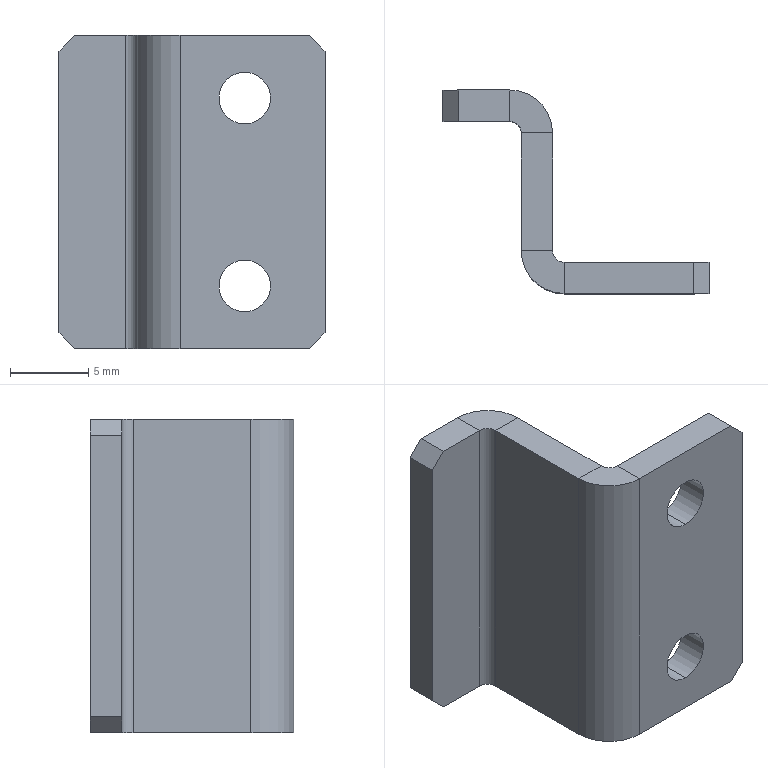Part | STEP file | 11-FG99-2015-7-17-S011-V3.0-kkkkkk-998.11 | 1 solid | 30 faces | box 17 x 13 x 20 mm | volume 1022 mm3 | plane 22 | cylinder 8 | commonest cylinder face diameters 3.3 x4 1.473 x2 5.473 x2
STEP:
#1=CARTESIAN_POINT('',(11.868,-11.,14.35));
#2=VERTEX_POINT('',#1);
#3=CARTESIAN_POINT('',(11.868,-11.,17.65));
#4=VERTEX_POINT('',#3);
#5=CARTESIAN_POINT('',(11.868,-11.,16.));
#6=DIRECTION('',(0.,1.,0.));
#7=DIRECTION('',(0.,0.,1.));
#8=AXIS2_PLACEMENT_3D('',#5,#6,#7);
#9=CIRCLE('',#8,1.65);
#10=EDGE_CURVE('',#2,#4,#9,.T.);
#11=ORIENTED_EDGE('',*,*,#10,.F.);
#12=CARTESIAN_POINT('',(11.868,-9.,14.35));
#13=VERTEX_POINT('',#12);
#14=CARTESIAN_POINT('',(11.868,-9.,14.35));
#15=DIRECTION('',(0.,1.,0.));
#16=VECTOR('',#15,1000.);
#17=LINE('',#14,#16);
#18=EDGE_CURVE('',#2,#13,#17,.T.);
#19=ORIENTED_EDGE('',*,*,#18,.T.);
#20=CARTESIAN_POINT('',(11.868,-9.,17.65));
#21=VERTEX_POINT('',#20);
#22=CARTESIAN_POINT('',(11.868,-9.,16.));
#23=DIRECTION('',(0.,1.,0.));
#24=DIRECTION('',(0.,0.,1.));
#25=AXIS2_PLACEMENT_3D('',#22,#23,#24);
#26=CIRCLE('',#25,1.65);
#27=EDGE_CURVE('',#13,#21,#26,.T.);
#28=ORIENTED_EDGE('',*,*,#27,.T.);
#29=CARTESIAN_POINT('',(11.868,-9.,17.65));
#30=DIRECTION('',(0.,1.,0.));
#31=VECTOR('',#30,1000.);
#32=LINE('',#29,#31);
#33=EDGE_CURVE('',#4,#21,#32,.T.);
#34=ORIENTED_EDGE('',*,*,#33,.F.);
#35=EDGE_LOOP('',(#11,#19,#28,#34));
#36=FACE_OUTER_BOUND('',#35,.T.);
#37=CARTESIAN_POINT('',(11.868,-9.,16.));
#38=DIRECTION('',(0.,1.,0.));
#39=DIRECTION('',(0.,0.,1.));
#40=AXIS2_PLACEMENT_3D('',#37,#38,#39);
#41=CYLINDRICAL_SURFACE('',#40,1.65);
#42=ADVANCED_FACE('',(#36),#41,.F.);
#43=CARTESIAN_POINT('',(11.868,-11.,2.35));
#44=VERTEX_POINT('',#43);
#45=CARTESIAN_POINT('',(11.868,-11.,5.65));
#46=VERTEX_POINT('',#45);
#47=CARTESIAN_POINT('',(11.868,-11.,4.));
#48=DIRECTION('',(0.,1.,0.));
#49=DIRECTION('',(0.,0.,1.));
#50=AXIS2_PLACEMENT_3D('',#47,#48,#49);
#51=CIRCLE('',#50,1.65);
#52=EDGE_CURVE('',#44,#46,#51,.T.);
#53=ORIENTED_EDGE('',*,*,#52,.F.);
#54=CARTESIAN_POINT('',(11.868,-9.,2.35));
#55=VERTEX_POINT('',#54);
#56=CARTESIAN_POINT('',(11.868,-9.,2.35));
#57=DIRECTION('',(0.,1.,0.));
#58=VECTOR('',#57,1000.);
#59=LINE('',#56,#58);
#60=EDGE_CURVE('',#44,#55,#59,.T.);
#61=ORIENTED_EDGE('',*,*,#60,.T.);
#62=CARTESIAN_POINT('',(11.868,-9.,5.65));
#63=VERTEX_POINT('',#62);
#64=CARTESIAN_POINT('',(11.868,-9.,4.));
#65=DIRECTION('',(0.,1.,0.));
#66=DIRECTION('',(0.,0.,1.));
#67=AXIS2_PLACEMENT_3D('',#64,#65,#66);
#68=CIRCLE('',#67,1.65);
#69=EDGE_CURVE('',#55,#63,#68,.T.);
#70=ORIENTED_EDGE('',*,*,#69,.T.);
#71=CARTESIAN_POINT('',(11.868,-9.,5.65));
#72=DIRECTION('',(0.,1.,0.));
#73=VECTOR('',#72,1000.);
#74=LINE('',#71,#73);
#75=EDGE_CURVE('',#46,#63,#74,.T.);
#76=ORIENTED_EDGE('',*,*,#75,.F.);
#77=EDGE_LOOP('',(#53,#61,#70,#76));
#78=FACE_OUTER_BOUND('',#77,.T.);
#79=CARTESIAN_POINT('',(11.868,-9.,4.));
#80=DIRECTION('',(0.,1.,0.));
#81=DIRECTION('',(0.,0.,1.));
#82=AXIS2_PLACEMENT_3D('',#79,#80,#81);
#83=CYLINDRICAL_SURFACE('',#82,1.65);
#84=ADVANCED_FACE('',(#78),#83,.F.);
#85=CARTESIAN_POINT('',(4.263,0.,20.));
#86=VERTEX_POINT('',#85);
#87=CARTESIAN_POINT('',(4.263,2.,20.));
#88=VERTEX_POINT('',#87);
#89=CARTESIAN_POINT('',(4.263,0.,20.));
#90=DIRECTION('',(0.,1.,0.));
#91=VECTOR('',#90,1000.);
#92=LINE('',#89,#91);
#93=EDGE_CURVE('',#86,#88,#92,.T.);
#94=ORIENTED_EDGE('',*,*,#93,.F.);
#95=CARTESIAN_POINT('',(5.,-0.7366,20.));
#96=VERTEX_POINT('',#95);
#97=CARTESIAN_POINT('',(4.263,-0.7366,20.));
#98=DIRECTION('',(0.,0.,-1.));
#99=DIRECTION('',(1.,0.,0.));
#100=AXIS2_PLACEMENT_3D('',#97,#98,#99);
#101=CIRCLE('',#100,0.7366);
#102=EDGE_CURVE('',#86,#96,#101,.T.);
#103=ORIENTED_EDGE('',*,*,#102,.T.);
#104=CARTESIAN_POINT('',(7.,-0.7366,20.));
#105=VERTEX_POINT('',#104);
#106=CARTESIAN_POINT('',(7.,-0.7366,20.));
#107=DIRECTION('',(-1.,0.,0.));
#108=VECTOR('',#107,1000.);
#109=LINE('',#106,#108);
#110=EDGE_CURVE('',#105,#96,#109,.T.);
#111=ORIENTED_EDGE('',*,*,#110,.F.);
#112=CARTESIAN_POINT('',(4.263,-0.7366,20.));
#113=DIRECTION('',(0.,0.,-1.));
#114=DIRECTION('',(1.,0.,0.));
#115=AXIS2_PLACEMENT_3D('',#112,#113,#114);
#116=CIRCLE('',#115,2.737);
#117=EDGE_CURVE('',#88,#105,#116,.T.);
#118=ORIENTED_EDGE('',*,*,#117,.F.);
#119=EDGE_LOOP('',(#94,#103,#111,#118));
#120=FACE_OUTER_BOUND('',#119,.T.);
#121=CARTESIAN_POINT('',(4.263,0.,20.));
#122=DIRECTION('',(0.,0.,1.));
#123=DIRECTION('',(1.,0.,0.));
#124=AXIS2_PLACEMENT_3D('',#121,#122,#123);
#125=PLANE('',#124);
#126=ADVANCED_FACE('',(#120),#125,.T.);
#127=CARTESIAN_POINT('',(1.,2.,20.));
#128=VERTEX_POINT('',#127);
#129=CARTESIAN_POINT('',(0.,2.,20.));
#130=DIRECTION('',(1.,0.,0.));
#131=VECTOR('',#130,1000.);
#132=LINE('',#129,#131);
#133=EDGE_CURVE('',#128,#88,#132,.T.);
#134=ORIENTED_EDGE('',*,*,#133,.F.);
#135=CARTESIAN_POINT('',(1.,0.,20.));
#136=VERTEX_POINT('',#135);
#137=CARTESIAN_POINT('',(1.,-0.7366,20.));
#138=DIRECTION('',(0.,-1.,0.));
#139=VECTOR('',#138,1000.);
#140=LINE('',#137,#139);
#141=EDGE_CURVE('',#128,#136,#140,.T.);
#142=ORIENTED_EDGE('',*,*,#141,.T.);
#143=CARTESIAN_POINT('',(0.,0.,20.));
#144=DIRECTION('',(1.,0.,0.));
#145=VECTOR('',#144,1000.);
#146=LINE('',#143,#145);
#147=EDGE_CURVE('',#136,#86,#146,.T.);
#148=ORIENTED_EDGE('',*,*,#147,.T.);
#149=ORIENTED_EDGE('',*,*,#93,.T.);
#150=EDGE_LOOP('',(#134,#142,#148,#149));
#151=FACE_OUTER_BOUND('',#150,.T.);
#152=CARTESIAN_POINT('',(7.,-0.7366,20.));
#153=DIRECTION('',(0.,0.,1.));
#154=DIRECTION('',(1.,0.,0.));
#155=AXIS2_PLACEMENT_3D('',#152,#153,#154);
#156=PLANE('',#155);
#157=ADVANCED_FACE('',(#151),#156,.T.);
#158=CARTESIAN_POINT('',(5.,-0.7366,0.));
#159=VERTEX_POINT('',#158);
#160=CARTESIAN_POINT('',(7.,-0.7366,0.));
#161=VERTEX_POINT('',#160);
#162=CARTESIAN_POINT('',(5.,-0.7366,0.));
#163=DIRECTION('',(1.,0.,0.));
#164=VECTOR('',#163,1000.);
#165=LINE('',#162,#164);
#166=EDGE_CURVE('',#159,#161,#165,.T.);
#167=ORIENTED_EDGE('',*,*,#166,.F.);
#168=CARTESIAN_POINT('',(4.263,0.,0.));
#169=VERTEX_POINT('',#168);
#170=CARTESIAN_POINT('',(4.263,-0.7366,0.));
#171=DIRECTION('',(0.,0.,-1.));
#172=DIRECTION('',(1.,0.,0.));
#173=AXIS2_PLACEMENT_3D('',#170,#171,#172);
#174=CIRCLE('',#173,0.7366);
#175=EDGE_CURVE('',#169,#159,#174,.T.);
#176=ORIENTED_EDGE('',*,*,#175,.F.);
#177=CARTESIAN_POINT('',(4.263,2.,0.));
#178=VERTEX_POINT('',#177);
#179=CARTESIAN_POINT('',(4.263,2.,0.));
#180=DIRECTION('',(0.,-1.,0.));
#181=VECTOR('',#180,1000.);
#182=LINE('',#179,#181);
#183=EDGE_CURVE('',#178,#169,#182,.T.);
#184=ORIENTED_EDGE('',*,*,#183,.F.);
#185=CARTESIAN_POINT('',(4.263,-0.7366,0.));
#186=DIRECTION('',(0.,0.,-1.));
#187=DIRECTION('',(1.,0.,0.));
#188=AXIS2_PLACEMENT_3D('',#185,#186,#187);
#189=CIRCLE('',#188,2.737);
#190=EDGE_CURVE('',#178,#161,#189,.T.);
#191=ORIENTED_EDGE('',*,*,#190,.T.);
#192=EDGE_LOOP('',(#167,#176,#184,#191));
#193=FACE_OUTER_BOUND('',#192,.T.);
#194=CARTESIAN_POINT('',(5.,-0.7366,0.));
#195=DIRECTION('',(0.,0.,-1.));
#196=DIRECTION('',(-1.,0.,0.));
#197=AXIS2_PLACEMENT_3D('',#194,#195,#196);
#198=PLANE('',#197);
#199=ADVANCED_FACE('',(#193),#198,.T.);
#200=CARTESIAN_POINT('',(5.,-8.263,0.));
#201=VERTEX_POINT('',#200);
#202=CARTESIAN_POINT('',(5.,0.,0.));
#203=DIRECTION('',(0.,-1.,0.));
#204=VECTOR('',#203,1000.);
#205=LINE('',#202,#204);
#206=EDGE_CURVE('',#159,#201,#205,.T.);
#207=ORIENTED_EDGE('',*,*,#206,.F.);
#208=ORIENTED_EDGE('',*,*,#166,.T.);
#209=CARTESIAN_POINT('',(7.,-8.263,0.));
#210=VERTEX_POINT('',#209);
#211=CARTESIAN_POINT('',(7.,0.,0.));
#212=DIRECTION('',(0.,-1.,0.));
#213=VECTOR('',#212,1000.);
#214=LINE('',#211,#213);
#215=EDGE_CURVE('',#161,#210,#214,.T.);
#216=ORIENTED_EDGE('',*,*,#215,.T.);
#217=CARTESIAN_POINT('',(7.,-8.263,0.));
#218=DIRECTION('',(-1.,0.,0.));
#219=VECTOR('',#218,1000.);
#220=LINE('',#217,#219);
#221=EDGE_CURVE('',#210,#201,#220,.T.);
#222=ORIENTED_EDGE('',*,*,#221,.T.);
#223=EDGE_LOOP('',(#207,#208,#216,#222));
#224=FACE_OUTER_BOUND('',#223,.T.);
#225=CARTESIAN_POINT('',(4.263,2.,0.));
#226=DIRECTION('',(0.,0.,-1.));
#227=DIRECTION('',(-1.,0.,0.));
#228=AXIS2_PLACEMENT_3D('',#225,#226,#227);
#229=PLANE('',#228);
#230=ADVANCED_FACE('',(#224),#229,.T.);
#231=CARTESIAN_POINT('',(5.,-8.263,20.));
#232=VERTEX_POINT('',#231);
#233=CARTESIAN_POINT('',(7.,-8.263,20.));
#234=VERTEX_POINT('',#233);
#235=CARTESIAN_POINT('',(5.,-8.263,20.));
#236=DIRECTION('',(1.,0.,0.));
#237=VECTOR('',#236,1000.);
#238=LINE('',#235,#237);
#239=EDGE_CURVE('',#232,#234,#238,.T.);
#240=ORIENTED_EDGE('',*,*,#239,.F.);
#241=CARTESIAN_POINT('',(7.737,-11.,20.));
#242=VERTEX_POINT('',#241);
#243=CARTESIAN_POINT('',(7.737,-8.263,20.));
#244=DIRECTION('',(0.,0.,1.));
#245=DIRECTION('',(-1.,0.,0.));
#246=AXIS2_PLACEMENT_3D('',#243,#244,#245);
#247=CIRCLE('',#246,2.737);
#248=EDGE_CURVE('',#232,#242,#247,.T.);
#249=ORIENTED_EDGE('',*,*,#248,.T.);
#250=CARTESIAN_POINT('',(7.737,-9.,20.));
#251=VERTEX_POINT('',#250);
#252=CARTESIAN_POINT('',(7.737,-9.,20.));
#253=DIRECTION('',(0.,-1.,0.));
#254=VECTOR('',#253,1000.);
#255=LINE('',#252,#254);
#256=EDGE_CURVE('',#251,#242,#255,.T.);
#257=ORIENTED_EDGE('',*,*,#256,.F.);
#258=CARTESIAN_POINT('',(7.737,-8.263,20.));
#259=DIRECTION('',(0.,0.,1.));
#260=DIRECTION('',(1.,0.,0.));
#261=AXIS2_PLACEMENT_3D('',#258,#259,#260);
#262=CIRCLE('',#261,0.7366);
#263=EDGE_CURVE('',#234,#251,#262,.T.);
#264=ORIENTED_EDGE('',*,*,#263,.F.);
#265=EDGE_LOOP('',(#240,#249,#257,#264));
#266=FACE_OUTER_BOUND('',#265,.T.);
#267=CARTESIAN_POINT('',(5.,-8.263,20.));
#268=DIRECTION('',(0.,0.,1.));
#269=DIRECTION('',(1.,0.,0.));
#270=AXIS2_PLACEMENT_3D('',#267,#268,#269);
#271=PLANE('',#270);
#272=ADVANCED_FACE('',(#266),#271,.T.);
#273=CARTESIAN_POINT('',(5.,0.,20.));
#274=DIRECTION('',(0.,-1.,0.));
#275=VECTOR('',#274,1000.);
#276=LINE('',#273,#275);
#277=EDGE_CURVE('',#96,#232,#276,.T.);
#278=ORIENTED_EDGE('',*,*,#277,.T.);
#279=ORIENTED_EDGE('',*,*,#239,.T.);
#280=CARTESIAN_POINT('',(7.,0.,20.));
#281=DIRECTION('',(0.,-1.,0.));
#282=VECTOR('',#281,1000.);
#283=LINE('',#280,#282);
#284=EDGE_CURVE('',#105,#234,#283,.T.);
#285=ORIENTED_EDGE('',*,*,#284,.F.);
#286=ORIENTED_EDGE('',*,*,#110,.T.);
#287=EDGE_LOOP('',(#278,#279,#285,#286));
#288=FACE_OUTER_BOUND('',#287,.T.);
#289=CARTESIAN_POINT('',(7.737,-9.,20.));
#290=DIRECTION('',(0.,0.,1.));
#291=DIRECTION('',(1.,0.,0.));
#292=AXIS2_PLACEMENT_3D('',#289,#290,#291);
#293=PLANE('',#292);
#294=ADVANCED_FACE('',(#288),#293,.T.);
#295=CARTESIAN_POINT('',(7.737,-11.,0.));
#296=VERTEX_POINT('',#295);
#297=CARTESIAN_POINT('',(7.737,-9.,0.));
#298=VERTEX_POINT('',#297);
#299=CARTESIAN_POINT('',(7.737,-11.,0.));
#300=DIRECTION('',(0.,1.,0.));
#301=VECTOR('',#300,1000.);
#302=LINE('',#299,#301);
#303=EDGE_CURVE('',#296,#298,#302,.T.);
#304=ORIENTED_EDGE('',*,*,#303,.F.);
#305=CARTESIAN_POINT('',(7.737,-8.263,0.));
#306=DIRECTION('',(0.,0.,1.));
#307=DIRECTION('',(-1.,0.,0.));
#308=AXIS2_PLACEMENT_3D('',#305,#306,#307);
#309=CIRCLE('',#308,2.737);
#310=EDGE_CURVE('',#201,#296,#309,.T.);
#311=ORIENTED_EDGE('',*,*,#310,.F.);
#312=ORIENTED_EDGE('',*,*,#221,.F.);
#313=CARTESIAN_POINT('',(7.737,-8.263,0.));
#314=DIRECTION('',(0.,0.,1.));
#315=DIRECTION('',(1.,0.,0.));
#316=AXIS2_PLACEMENT_3D('',#313,#314,#315);
#317=CIRCLE('',#316,0.7366);
#318=EDGE_CURVE('',#210,#298,#317,.T.);
#319=ORIENTED_EDGE('',*,*,#318,.T.);
#320=EDGE_LOOP('',(#304,#311,#312,#319));
#321=FACE_OUTER_BOUND('',#320,.T.);
#322=CARTESIAN_POINT('',(7.737,-11.,0.));
#323=DIRECTION('',(0.,0.,-1.));
#324=DIRECTION('',(-1.,0.,0.));
#325=AXIS2_PLACEMENT_3D('',#322,#323,#324);
#326=PLANE('',#325);
#327=ADVANCED_FACE('',(#321),#326,.T.);
#328=CARTESIAN_POINT('',(16.,-9.,0.));
#329=VERTEX_POINT('',#328);
#330=CARTESIAN_POINT('',(5.,-9.,0.));
#331=DIRECTION('',(1.,0.,0.));
#332=VECTOR('',#331,1000.);
#333=LINE('',#330,#332);
#334=EDGE_CURVE('',#298,#329,#333,.T.);
#335=ORIENTED_EDGE('',*,*,#334,.T.);
#336=CARTESIAN_POINT('',(16.,-11.,0.));
#337=VERTEX_POINT('',#336);
#338=CARTESIAN_POINT('',(16.,-8.263,0.));
#339=DIRECTION('',(0.,-1.,0.));
#340=VECTOR('',#339,1000.);
#341=LINE('',#338,#340);
#342=EDGE_CURVE('',#329,#337,#341,.T.);
#343=ORIENTED_EDGE('',*,*,#342,.T.);
#344=CARTESIAN_POINT('',(5.,-11.,0.));
#345=DIRECTION('',(1.,0.,0.));
#346=VECTOR('',#345,1000.);
#347=LINE('',#344,#346);
#348=EDGE_CURVE('',#296,#337,#347,.T.);
#349=ORIENTED_EDGE('',*,*,#348,.F.);
#350=ORIENTED_EDGE('',*,*,#303,.T.);
#351=EDGE_LOOP('',(#335,#343,#349,#350));
#352=FACE_OUTER_BOUND('',#351,.T.);
#353=CARTESIAN_POINT('',(7.,-8.263,0.));
#354=DIRECTION('',(0.,0.,-1.));
#355=DIRECTION('',(-1.,0.,0.));
#356=AXIS2_PLACEMENT_3D('',#353,#354,#355);
#357=PLANE('',#356);
#358=ADVANCED_FACE('',(#352),#357,.T.);
#359=CARTESIAN_POINT('',(11.868,-11.,16.));
#360=DIRECTION('',(0.,1.,0.));
#361=DIRECTION('',(0.,0.,1.));
#362=AXIS2_PLACEMENT_3D('',#359,#360,#361);
#363=CIRCLE('',#362,1.65);
#364=EDGE_CURVE('',#4,#2,#363,.T.);
#365=ORIENTED_EDGE('',*,*,#364,.T.);
#366=ORIENTED_EDGE('',*,*,#10,.T.);
#367=EDGE_LOOP('',(#365,#366));
#368=FACE_BOUND('',#367,.T.);
#369=CARTESIAN_POINT('',(11.868,-11.,4.));
#370=DIRECTION('',(0.,1.,0.));
#371=DIRECTION('',(0.,0.,1.));
#372=AXIS2_PLACEMENT_3D('',#369,#370,#371);
#373=CIRCLE('',#372,1.65);
#374=EDGE_CURVE('',#46,#44,#373,.T.);
#375=ORIENTED_EDGE('',*,*,#374,.T.);
#376=ORIENTED_EDGE('',*,*,#52,.T.);
#377=EDGE_LOOP('',(#375,#376));
#378=FACE_BOUND('',#377,.T.);
#379=ORIENTED_EDGE('',*,*,#348,.T.);
#380=CARTESIAN_POINT('',(17.,-11.,1.));
#381=VERTEX_POINT('',#380);
#382=CARTESIAN_POINT('',(16.,-11.,0.));
#383=DIRECTION('',(0.7071,0.,0.7071));
#384=VECTOR('',#383,1000.);
#385=LINE('',#382,#384);
#386=EDGE_CURVE('',#337,#381,#385,.T.);
#387=ORIENTED_EDGE('',*,*,#386,.T.);
#388=CARTESIAN_POINT('',(17.,-11.,19.));
#389=VERTEX_POINT('',#388);
#390=CARTESIAN_POINT('',(17.,-11.,20.));
#391=DIRECTION('',(0.,0.,-1.));
#392=VECTOR('',#391,1000.);
#393=LINE('',#390,#392);
#394=EDGE_CURVE('',#389,#381,#393,.T.);
#395=ORIENTED_EDGE('',*,*,#394,.F.);
#396=CARTESIAN_POINT('',(16.,-11.,20.));
#397=VERTEX_POINT('',#396);
#398=CARTESIAN_POINT('',(17.,-11.,19.));
#399=DIRECTION('',(-0.7071,0.,0.7071));
#400=VECTOR('',#399,1000.);
#401=LINE('',#398,#400);
#402=EDGE_CURVE('',#389,#397,#401,.T.);
#403=ORIENTED_EDGE('',*,*,#402,.T.);
#404=CARTESIAN_POINT('',(5.,-11.,20.));
#405=DIRECTION('',(1.,0.,0.));
#406=VECTOR('',#405,1000.);
#407=LINE('',#404,#406);
#408=EDGE_CURVE('',#242,#397,#407,.T.);
#409=ORIENTED_EDGE('',*,*,#408,.F.);
#410=CARTESIAN_POINT('',(7.737,-11.,20.));
#411=DIRECTION('',(0.,0.,-1.));
#412=VECTOR('',#411,1000.);
#413=LINE('',#410,#412);
#414=EDGE_CURVE('',#242,#296,#413,.T.);
#415=ORIENTED_EDGE('',*,*,#414,.T.);
#416=EDGE_LOOP('',(#379,#387,#395,#403,#409,#415));
#417=FACE_OUTER_BOUND('',#416,.T.);
#418=CARTESIAN_POINT('',(5.,-11.,20.));
#419=DIRECTION('',(0.,1.,0.));
#420=DIRECTION('',(0.,0.,1.));
#421=AXIS2_PLACEMENT_3D('',#418,#419,#420);
#422=PLANE('',#421);
#423=ADVANCED_FACE('',(#368,#378,#417),#422,.F.);
#424=ORIENTED_EDGE('',*,*,#394,.T.);
#425=CARTESIAN_POINT('',(17.,-9.,1.));
#426=VERTEX_POINT('',#425);
#427=CARTESIAN_POINT('',(17.,-9.,1.));
#428=DIRECTION('',(0.,1.,0.));
#429=VECTOR('',#428,1000.);
#430=LINE('',#427,#429);
#431=EDGE_CURVE('',#381,#426,#430,.T.);
#432=ORIENTED_EDGE('',*,*,#431,.T.);
#433=CARTESIAN_POINT('',(17.,-9.,19.));
#434=VERTEX_POINT('',#433);
#435=CARTESIAN_POINT('',(17.,-9.,20.));
#436=DIRECTION('',(0.,0.,-1.));
#437=VECTOR('',#436,1000.);
#438=LINE('',#435,#437);
#439=EDGE_CURVE('',#434,#426,#438,.T.);
#440=ORIENTED_EDGE('',*,*,#439,.F.);
#441=CARTESIAN_POINT('',(17.,-9.,19.));
#442=DIRECTION('',(0.,-1.,0.));
#443=VECTOR('',#442,1000.);
#444=LINE('',#441,#443);
#445=EDGE_CURVE('',#434,#389,#444,.T.);
#446=ORIENTED_EDGE('',*,*,#445,.T.);
#447=EDGE_LOOP('',(#424,#432,#440,#446));
#448=FACE_OUTER_BOUND('',#447,.T.);
#449=CARTESIAN_POINT('',(17.,-9.,20.));
#450=DIRECTION('',(1.,0.,0.));
#451=DIRECTION('',(0.,0.,-1.));
#452=AXIS2_PLACEMENT_3D('',#449,#450,#451);
#453=PLANE('',#452);
#454=ADVANCED_FACE('',(#448),#453,.T.);
#455=CARTESIAN_POINT('',(11.868,-9.,16.));
#456=DIRECTION('',(0.,1.,0.));
#457=DIRECTION('',(0.,0.,1.));
#458=AXIS2_PLACEMENT_3D('',#455,#456,#457);
#459=CIRCLE('',#458,1.65);
#460=EDGE_CURVE('',#21,#13,#459,.T.);
#461=ORIENTED_EDGE('',*,*,#460,.F.);
#462=ORIENTED_EDGE('',*,*,#27,.F.);
#463=EDGE_LOOP('',(#461,#462));
#464=FACE_BOUND('',#463,.T.);
#465=CARTESIAN_POINT('',(11.868,-9.,4.));
#466=DIRECTION('',(0.,1.,0.));
#467=DIRECTION('',(0.,0.,1.));
#468=AXIS2_PLACEMENT_3D('',#465,#466,#467);
#469=CIRCLE('',#468,1.65);
#470=EDGE_CURVE('',#63,#55,#469,.T.);
#471=ORIENTED_EDGE('',*,*,#470,.F.);
#472=ORIENTED_EDGE('',*,*,#69,.F.);
#473=EDGE_LOOP('',(#471,#472));
#474=FACE_BOUND('',#473,.T.);
#475=ORIENTED_EDGE('',*,*,#439,.T.);
#476=CARTESIAN_POINT('',(20.5,-9.,4.5));
#477=DIRECTION('',(-0.7071,0.,-0.7071));
#478=VECTOR('',#477,1000.);
#479=LINE('',#476,#478);
#480=EDGE_CURVE('',#426,#329,#479,.T.);
#481=ORIENTED_EDGE('',*,*,#480,.T.);
#482=ORIENTED_EDGE('',*,*,#334,.F.);
#483=CARTESIAN_POINT('',(7.737,-9.,20.));
#484=DIRECTION('',(0.,0.,-1.));
#485=VECTOR('',#484,1000.);
#486=LINE('',#483,#485);
#487=EDGE_CURVE('',#251,#298,#486,.T.);
#488=ORIENTED_EDGE('',*,*,#487,.F.);
#489=CARTESIAN_POINT('',(16.,-9.,20.));
#490=VERTEX_POINT('',#489);
#491=CARTESIAN_POINT('',(5.,-9.,20.));
#492=DIRECTION('',(1.,0.,0.));
#493=VECTOR('',#492,1000.);
#494=LINE('',#491,#493);
#495=EDGE_CURVE('',#251,#490,#494,.T.);
#496=ORIENTED_EDGE('',*,*,#495,.T.);
#497=CARTESIAN_POINT('',(10.5,-9.,25.5));
#498=DIRECTION('',(0.7071,0.,-0.7071));
#499=VECTOR('',#498,1000.);
#500=LINE('',#497,#499);
#501=EDGE_CURVE('',#490,#434,#500,.T.);
#502=ORIENTED_EDGE('',*,*,#501,.T.);
#503=EDGE_LOOP('',(#475,#481,#482,#488,#496,#502));
#504=FACE_OUTER_BOUND('',#503,.T.);
#505=CARTESIAN_POINT('',(5.,-9.,20.));
#506=DIRECTION('',(0.,1.,0.));
#507=DIRECTION('',(0.,0.,1.));
#508=AXIS2_PLACEMENT_3D('',#505,#506,#507);
#509=PLANE('',#508);
#510=ADVANCED_FACE('',(#464,#474,#504),#509,.T.);
#511=ORIENTED_EDGE('',*,*,#318,.F.);
#512=CARTESIAN_POINT('',(7.,-8.263,20.));
#513=DIRECTION('',(0.,0.,-1.));
#514=VECTOR('',#513,1000.);
#515=LINE('',#512,#514);
#516=EDGE_CURVE('',#234,#210,#515,.T.);
#517=ORIENTED_EDGE('',*,*,#516,.F.);
#518=ORIENTED_EDGE('',*,*,#263,.T.);
#519=ORIENTED_EDGE('',*,*,#487,.T.);
#520=EDGE_LOOP('',(#511,#517,#518,#519));
#521=FACE_OUTER_BOUND('',#520,.T.);
#522=CARTESIAN_POINT('',(7.737,-8.263,20.));
#523=DIRECTION('',(0.,0.,-1.));
#524=DIRECTION('',(-1.,0.,0.));
#525=AXIS2_PLACEMENT_3D('',#522,#523,#524);
#526=CYLINDRICAL_SURFACE('',#525,0.7366);
#527=ADVANCED_FACE('',(#521),#526,.F.);
#528=ORIENTED_EDGE('',*,*,#215,.F.);
#529=CARTESIAN_POINT('',(7.,-0.7366,20.));
#530=DIRECTION('',(0.,0.,-1.));
#531=VECTOR('',#530,1000.);
#532=LINE('',#529,#531);
#533=EDGE_CURVE('',#105,#161,#532,.T.);
#534=ORIENTED_EDGE('',*,*,#533,.F.);
#535=ORIENTED_EDGE('',*,*,#284,.T.);
#536=ORIENTED_EDGE('',*,*,#516,.T.);
#537=EDGE_LOOP('',(#528,#534,#535,#536));
#538=FACE_OUTER_BOUND('',#537,.T.);
#539=CARTESIAN_POINT('',(7.,0.,20.));
#540=DIRECTION('',(1.,0.,0.));
#541=DIRECTION('',(0.,1.,0.));
#542=AXIS2_PLACEMENT_3D('',#539,#540,#541);
#543=PLANE('',#542);
#544=ADVANCED_FACE('',(#538),#543,.T.);
#545=ORIENTED_EDGE('',*,*,#190,.F.);
#546=CARTESIAN_POINT('',(4.263,2.,20.));
#547=DIRECTION('',(0.,0.,-1.));
#548=VECTOR('',#547,1000.);
#549=LINE('',#546,#548);
#550=EDGE_CURVE('',#88,#178,#549,.T.);
#551=ORIENTED_EDGE('',*,*,#550,.F.);
#552=ORIENTED_EDGE('',*,*,#117,.T.);
#553=ORIENTED_EDGE('',*,*,#533,.T.);
#554=EDGE_LOOP('',(#545,#551,#552,#553));
#555=FACE_OUTER_BOUND('',#554,.T.);
#556=CARTESIAN_POINT('',(4.263,-0.7366,20.));
#557=DIRECTION('',(0.,0.,-1.));
#558=DIRECTION('',(-1.,0.,0.));
#559=AXIS2_PLACEMENT_3D('',#556,#557,#558);
#560=CYLINDRICAL_SURFACE('',#559,2.737);
#561=ADVANCED_FACE('',(#555),#560,.T.);
#562=CARTESIAN_POINT('',(1.,2.,0.));
#563=VERTEX_POINT('',#562);
#564=CARTESIAN_POINT('',(0.,2.,0.));
#565=DIRECTION('',(1.,0.,0.));
#566=VECTOR('',#565,1000.);
#567=LINE('',#564,#566);
#568=EDGE_CURVE('',#563,#178,#567,.T.);
#569=ORIENTED_EDGE('',*,*,#568,.F.);
#570=CARTESIAN_POINT('',(0.,2.,1.));
#571=VERTEX_POINT('',#570);
#572=CARTESIAN_POINT('',(-9.5,2.,10.5));
#573=DIRECTION('',(-0.7071,0.,0.7071));
#574=VECTOR('',#573,1000.);
#575=LINE('',#572,#574);
#576=EDGE_CURVE('',#563,#571,#575,.T.);
#577=ORIENTED_EDGE('',*,*,#576,.T.);
#578=CARTESIAN_POINT('',(0.,2.,19.));
#579=VERTEX_POINT('',#578);
#580=CARTESIAN_POINT('',(0.,2.,20.));
#581=DIRECTION('',(0.,0.,-1.));
#582=VECTOR('',#581,1000.);
#583=LINE('',#580,#582);
#584=EDGE_CURVE('',#579,#571,#583,.T.);
#585=ORIENTED_EDGE('',*,*,#584,.F.);
#586=CARTESIAN_POINT('',(0.5,2.,19.5));
#587=DIRECTION('',(0.7071,0.,0.7071));
#588=VECTOR('',#587,1000.);
#589=LINE('',#586,#588);
#590=EDGE_CURVE('',#579,#128,#589,.T.);
#591=ORIENTED_EDGE('',*,*,#590,.T.);
#592=ORIENTED_EDGE('',*,*,#133,.T.);
#593=ORIENTED_EDGE('',*,*,#550,.T.);
#594=EDGE_LOOP('',(#569,#577,#585,#591,#592,#593));
#595=FACE_OUTER_BOUND('',#594,.T.);
#596=CARTESIAN_POINT('',(0.,2.,20.));
#597=DIRECTION('',(0.,1.,0.));
#598=DIRECTION('',(0.,0.,1.));
#599=AXIS2_PLACEMENT_3D('',#596,#597,#598);
#600=PLANE('',#599);
#601=ADVANCED_FACE('',(#595),#600,.T.);
#602=ORIENTED_EDGE('',*,*,#584,.T.);
#603=CARTESIAN_POINT('',(0.,0.,1.));
#604=VERTEX_POINT('',#603);
#605=CARTESIAN_POINT('',(0.,0.,1.));
#606=DIRECTION('',(0.,-1.,0.));
#607=VECTOR('',#606,1000.);
#608=LINE('',#605,#607);
#609=EDGE_CURVE('',#571,#604,#608,.T.);
#610=ORIENTED_EDGE('',*,*,#609,.T.);
#611=CARTESIAN_POINT('',(0.,0.,19.));
#612=VERTEX_POINT('',#611);
#613=CARTESIAN_POINT('',(0.,0.,20.));
#614=DIRECTION('',(0.,0.,-1.));
#615=VECTOR('',#614,1000.);
#616=LINE('',#613,#615);
#617=EDGE_CURVE('',#612,#604,#616,.T.);
#618=ORIENTED_EDGE('',*,*,#617,.F.);
#619=CARTESIAN_POINT('',(0.,0.,19.));
#620=DIRECTION('',(0.,1.,0.));
#621=VECTOR('',#620,1000.);
#622=LINE('',#619,#621);
#623=EDGE_CURVE('',#612,#579,#622,.T.);
#624=ORIENTED_EDGE('',*,*,#623,.T.);
#625=EDGE_LOOP('',(#602,#610,#618,#624));
#626=FACE_OUTER_BOUND('',#625,.T.);
#627=CARTESIAN_POINT('',(0.,0.,20.));
#628=DIRECTION('',(-1.,0.,0.));
#629=DIRECTION('',(0.,0.,1.));
#630=AXIS2_PLACEMENT_3D('',#627,#628,#629);
#631=PLANE('',#630);
#632=ADVANCED_FACE('',(#626),#631,.T.);
#633=ORIENTED_EDGE('',*,*,#617,.T.);
#634=CARTESIAN_POINT('',(1.,0.,0.));
#635=VERTEX_POINT('',#634);
#636=CARTESIAN_POINT('',(1.,0.,0.));
#637=DIRECTION('',(0.7071,0.,-0.7071));
#638=VECTOR('',#637,1000.);
#639=LINE('',#636,#638);
#640=EDGE_CURVE('',#604,#635,#639,.T.);
#641=ORIENTED_EDGE('',*,*,#640,.T.);
#642=CARTESIAN_POINT('',(0.,0.,0.));
#643=DIRECTION('',(1.,0.,0.));
#644=VECTOR('',#643,1000.);
#645=LINE('',#642,#644);
#646=EDGE_CURVE('',#635,#169,#645,.T.);
#647=ORIENTED_EDGE('',*,*,#646,.T.);
#648=CARTESIAN_POINT('',(4.263,0.,20.));
#649=DIRECTION('',(0.,0.,-1.));
#650=VECTOR('',#649,1000.);
#651=LINE('',#648,#650);
#652=EDGE_CURVE('',#86,#169,#651,.T.);
#653=ORIENTED_EDGE('',*,*,#652,.F.);
#654=ORIENTED_EDGE('',*,*,#147,.F.);
#655=CARTESIAN_POINT('',(0.,0.,19.));
#656=DIRECTION('',(-0.7071,0.,-0.7071));
#657=VECTOR('',#656,1000.);
#658=LINE('',#655,#657);
#659=EDGE_CURVE('',#136,#612,#658,.T.);
#660=ORIENTED_EDGE('',*,*,#659,.T.);
#661=EDGE_LOOP('',(#633,#641,#647,#653,#654,#660));
#662=FACE_OUTER_BOUND('',#661,.T.);
#663=CARTESIAN_POINT('',(0.,0.,20.));
#664=DIRECTION('',(0.,1.,0.));
#665=DIRECTION('',(0.,0.,1.));
#666=AXIS2_PLACEMENT_3D('',#663,#664,#665);
#667=PLANE('',#666);
#668=ADVANCED_FACE('',(#662),#667,.F.);
#669=ORIENTED_EDGE('',*,*,#175,.T.);
#670=CARTESIAN_POINT('',(5.,-0.7366,20.));
#671=DIRECTION('',(0.,0.,-1.));
#672=VECTOR('',#671,1000.);
#673=LINE('',#670,#672);
#674=EDGE_CURVE('',#96,#159,#673,.T.);
#675=ORIENTED_EDGE('',*,*,#674,.F.);
#676=ORIENTED_EDGE('',*,*,#102,.F.);
#677=ORIENTED_EDGE('',*,*,#652,.T.);
#678=EDGE_LOOP('',(#669,#675,#676,#677));
#679=FACE_OUTER_BOUND('',#678,.T.);
#680=CARTESIAN_POINT('',(4.263,-0.7366,20.));
#681=DIRECTION('',(0.,0.,-1.));
#682=DIRECTION('',(-1.,0.,0.));
#683=AXIS2_PLACEMENT_3D('',#680,#681,#682);
#684=CYLINDRICAL_SURFACE('',#683,0.7366);
#685=ADVANCED_FACE('',(#679),#684,.F.);
#686=ORIENTED_EDGE('',*,*,#206,.T.);
#687=CARTESIAN_POINT('',(5.,-8.263,20.));
#688=DIRECTION('',(0.,0.,-1.));
#689=VECTOR('',#688,1000.);
#690=LINE('',#687,#689);
#691=EDGE_CURVE('',#232,#201,#690,.T.);
#692=ORIENTED_EDGE('',*,*,#691,.F.);
#693=ORIENTED_EDGE('',*,*,#277,.F.);
#694=ORIENTED_EDGE('',*,*,#674,.T.);
#695=EDGE_LOOP('',(#686,#692,#693,#694));
#696=FACE_OUTER_BOUND('',#695,.T.);
#697=CARTESIAN_POINT('',(5.,0.,20.));
#698=DIRECTION('',(1.,0.,0.));
#699=DIRECTION('',(0.,1.,0.));
#700=AXIS2_PLACEMENT_3D('',#697,#698,#699);
#701=PLANE('',#700);
#702=ADVANCED_FACE('',(#696),#701,.F.);
#703=ORIENTED_EDGE('',*,*,#310,.T.);
#704=ORIENTED_EDGE('',*,*,#414,.F.);
#705=ORIENTED_EDGE('',*,*,#248,.F.);
#706=ORIENTED_EDGE('',*,*,#691,.T.);
#707=EDGE_LOOP('',(#703,#704,#705,#706));
#708=FACE_OUTER_BOUND('',#707,.T.);
#709=CARTESIAN_POINT('',(7.737,-8.263,20.));
#710=DIRECTION('',(0.,0.,-1.));
#711=DIRECTION('',(-1.,0.,0.));
#712=AXIS2_PLACEMENT_3D('',#709,#710,#711);
#713=CYLINDRICAL_SURFACE('',#712,2.737);
#714=ADVANCED_FACE('',(#708),#713,.T.);
#715=ORIENTED_EDGE('',*,*,#408,.T.);
#716=CARTESIAN_POINT('',(16.,-8.263,20.));
#717=DIRECTION('',(0.,1.,0.));
#718=VECTOR('',#717,1000.);
#719=LINE('',#716,#718);
#720=EDGE_CURVE('',#397,#490,#719,.T.);
#721=ORIENTED_EDGE('',*,*,#720,.T.);
#722=ORIENTED_EDGE('',*,*,#495,.F.);
#723=ORIENTED_EDGE('',*,*,#256,.T.);
#724=EDGE_LOOP('',(#715,#721,#722,#723));
#725=FACE_OUTER_BOUND('',#724,.T.);
#726=CARTESIAN_POINT('',(7.737,-8.263,20.));
#727=DIRECTION('',(0.,0.,1.));
#728=DIRECTION('',(1.,0.,0.));
#729=AXIS2_PLACEMENT_3D('',#726,#727,#728);
#730=PLANE('',#729);
#731=ADVANCED_FACE('',(#725),#730,.T.);
#732=ORIENTED_EDGE('',*,*,#646,.F.);
#733=CARTESIAN_POINT('',(1.,2.,0.));
#734=DIRECTION('',(0.,1.,0.));
#735=VECTOR('',#734,1000.);
#736=LINE('',#733,#735);
#737=EDGE_CURVE('',#635,#563,#736,.T.);
#738=ORIENTED_EDGE('',*,*,#737,.T.);
#739=ORIENTED_EDGE('',*,*,#568,.T.);
#740=ORIENTED_EDGE('',*,*,#183,.T.);
#741=EDGE_LOOP('',(#732,#738,#739,#740));
#742=FACE_OUTER_BOUND('',#741,.T.);
#743=CARTESIAN_POINT('',(7.737,-8.263,0.));
#744=DIRECTION('',(0.,0.,1.));
#745=DIRECTION('',(1.,0.,0.));
#746=AXIS2_PLACEMENT_3D('',#743,#744,#745);
#747=PLANE('',#746);
#748=ADVANCED_FACE('',(#742),#747,.F.);
#749=ORIENTED_EDGE('',*,*,#640,.F.);
#750=ORIENTED_EDGE('',*,*,#609,.F.);
#751=ORIENTED_EDGE('',*,*,#576,.F.);
#752=ORIENTED_EDGE('',*,*,#737,.F.);
#753=EDGE_LOOP('',(#749,#750,#751,#752));
#754=FACE_OUTER_BOUND('',#753,.T.);
#755=CARTESIAN_POINT('',(1.,-8.263,0.));
#756=DIRECTION('',(-0.7071,0.,-0.7071));
#757=DIRECTION('',(0.,-1.,0.));
#758=AXIS2_PLACEMENT_3D('',#755,#756,#757);
#759=PLANE('',#758);
#760=ADVANCED_FACE('',(#754),#759,.T.);
#761=ORIENTED_EDGE('',*,*,#659,.F.);
#762=ORIENTED_EDGE('',*,*,#141,.F.);
#763=ORIENTED_EDGE('',*,*,#590,.F.);
#764=ORIENTED_EDGE('',*,*,#623,.F.);
#765=EDGE_LOOP('',(#761,#762,#763,#764));
#766=FACE_OUTER_BOUND('',#765,.T.);
#767=CARTESIAN_POINT('',(0.,0.,19.));
#768=DIRECTION('',(0.7071,0.,-0.7071));
#769=DIRECTION('',(0.,1.,0.));
#770=AXIS2_PLACEMENT_3D('',#767,#768,#769);
#771=PLANE('',#770);
#772=ADVANCED_FACE('',(#766),#771,.F.);
#773=ORIENTED_EDGE('',*,*,#480,.F.);
#774=ORIENTED_EDGE('',*,*,#431,.F.);
#775=ORIENTED_EDGE('',*,*,#386,.F.);
#776=ORIENTED_EDGE('',*,*,#342,.F.);
#777=EDGE_LOOP('',(#773,#774,#775,#776));
#778=FACE_OUTER_BOUND('',#777,.T.);
#779=CARTESIAN_POINT('',(16.,-8.263,0.));
#780=DIRECTION('',(-0.7071,0.,0.7071));
#781=DIRECTION('',(0.,-1.,0.));
#782=AXIS2_PLACEMENT_3D('',#779,#780,#781);
#783=PLANE('',#782);
#784=ADVANCED_FACE('',(#778),#783,.F.);
#785=ORIENTED_EDGE('',*,*,#501,.F.);
#786=ORIENTED_EDGE('',*,*,#720,.F.);
#787=ORIENTED_EDGE('',*,*,#402,.F.);
#788=ORIENTED_EDGE('',*,*,#445,.F.);
#789=EDGE_LOOP('',(#785,#786,#787,#788));
#790=FACE_OUTER_BOUND('',#789,.T.);
#791=CARTESIAN_POINT('',(17.,-9.,19.));
#792=DIRECTION('',(-0.7071,0.,-0.7071));
#793=DIRECTION('',(0.,-1.,0.));
#794=AXIS2_PLACEMENT_3D('',#791,#792,#793);
#795=PLANE('',#794);
#796=ADVANCED_FACE('',(#790),#795,.F.);
#797=ORIENTED_EDGE('',*,*,#60,.F.);
#798=ORIENTED_EDGE('',*,*,#374,.F.);
#799=ORIENTED_EDGE('',*,*,#75,.T.);
#800=ORIENTED_EDGE('',*,*,#470,.T.);
#801=EDGE_LOOP('',(#797,#798,#799,#800));
#802=FACE_OUTER_BOUND('',#801,.T.);
#803=CARTESIAN_POINT('',(11.868,-9.,4.));
#804=DIRECTION('',(0.,1.,0.));
#805=DIRECTION('',(0.,0.,1.));
#806=AXIS2_PLACEMENT_3D('',#803,#804,#805);
#807=CYLINDRICAL_SURFACE('',#806,1.65);
#808=ADVANCED_FACE('',(#802),#807,.F.);
#809=ORIENTED_EDGE('',*,*,#18,.F.);
#810=ORIENTED_EDGE('',*,*,#364,.F.);
#811=ORIENTED_EDGE('',*,*,#33,.T.);
#812=ORIENTED_EDGE('',*,*,#460,.T.);
#813=EDGE_LOOP('',(#809,#810,#811,#812));
#814=FACE_OUTER_BOUND('',#813,.T.);
#815=CARTESIAN_POINT('',(11.868,-9.,16.));
#816=DIRECTION('',(0.,1.,0.));
#817=DIRECTION('',(0.,0.,1.));
#818=AXIS2_PLACEMENT_3D('',#815,#816,#817);
#819=CYLINDRICAL_SURFACE('',#818,1.65);
#820=ADVANCED_FACE('',(#814),#819,.F.);
#821=CLOSED_SHELL('',(#42,#84,#126,#157,#199,#230,#272,#294,#327,#358,#423,#454,#510,#527,#544,#561,#601,#632,#668,#685,#702,#714,#731,#748,#760,#772,#784,#796,#808,#820));
#822=MANIFOLD_SOLID_BREP('',#821);
#823=CARTESIAN_POINT('',(0.,0.,0.));
#824=DIRECTION('',(0.,0.,1.));
#825=DIRECTION('',(1.,0.,0.));
#826=AXIS2_PLACEMENT_3D('',#823,#824,#825);
#827=(LENGTH_UNIT()NAMED_UNIT(*)SI_UNIT(.MILLI.,.METRE.));
#828=UNCERTAINTY_MEASURE_WITH_UNIT(LENGTH_MEASURE(0.00001),#827,'','');
#829=(NAMED_UNIT(*)PLANE_ANGLE_UNIT()SI_UNIT($,.RADIAN.));
#830=(NAMED_UNIT(*)SI_UNIT($,.STERADIAN.)SOLID_ANGLE_UNIT());
#831=(GEOMETRIC_REPRESENTATION_CONTEXT(3)GLOBAL_UNCERTAINTY_ASSIGNED_CONTEXT((#828))GLOBAL_UNIT_ASSIGNED_CONTEXT((#827,#829,#830))REPRESENTATION_CONTEXT('',''));
#832=ADVANCED_BREP_SHAPE_REPRESENTATION('',(#822,#826),#831);